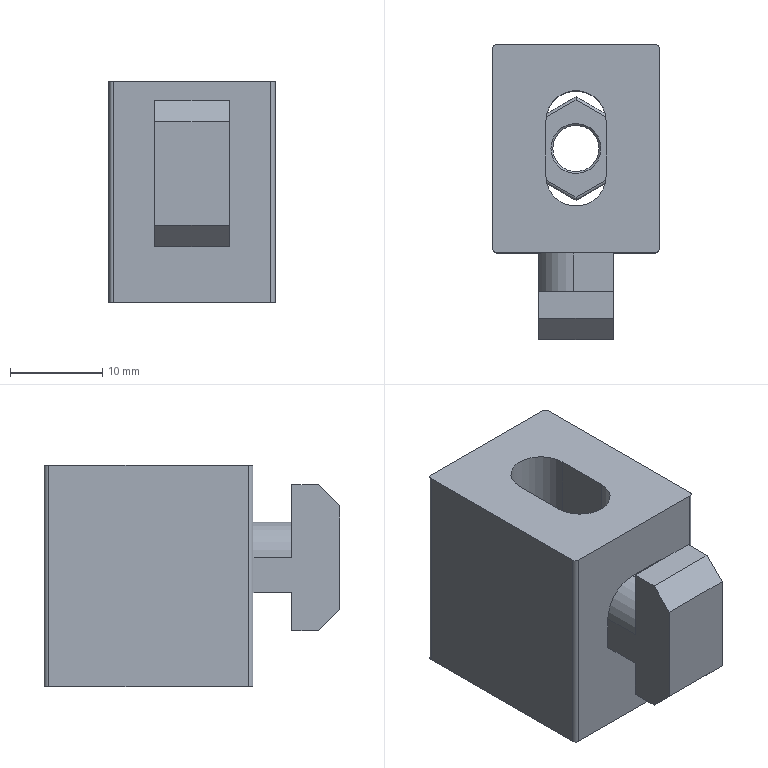Part | STEP file | spacer connection block MK-PMB-T-40 | 1 solid | 60 faces | box 18 x 32 x 24 mm | volume 8600 mm3 | plane 32 | cylinder 24 | cone 4 | commonest cylinder face diameters 0.6 x12 1 x4 6.5 x4 5 x2 7.6 x2